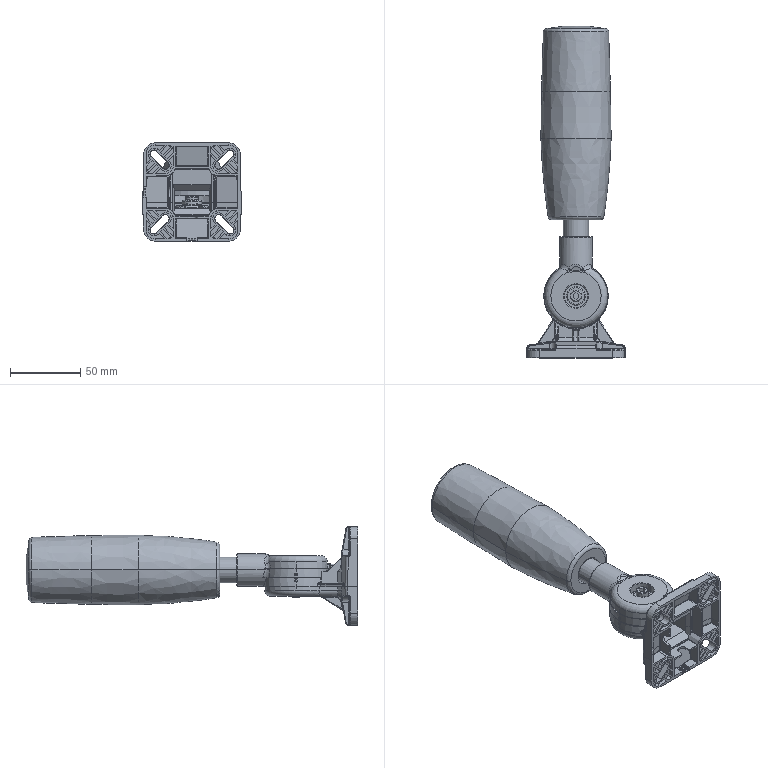Part | SolidWorks | features BaseBody 9 | 9 solids | 1618 faces | box 70 x 236.301 x 70 mm | volume 289384 mm3 | plane 538 | cylinder 464 | spline 200 | cone 183 | torus 182 | sphere 51 | commonest cylinder face diameters 1 x150 0.6 x70 4.85 x62 0.4 x44 0.2 x20 4 x15